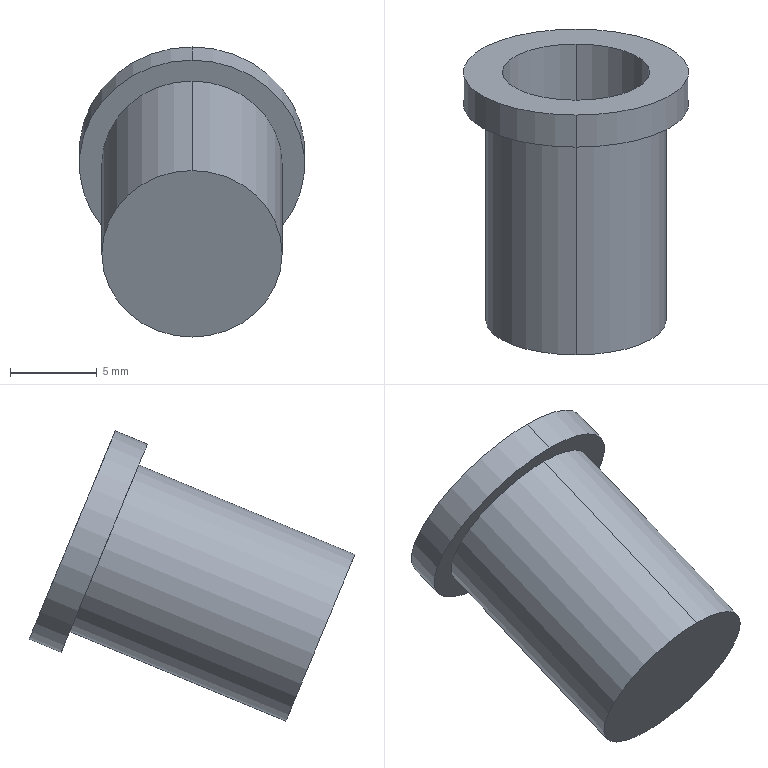Part | STEP file | ADMI9201SOYF_11_1 | 1 solid | 10 faces | box 13 x 18.798 x 16.741 mm | volume 788.076 mm3 | cylinder 6 | plane 4 | commonest cylinder face diameters 8.5 x2 10.4 x2 13 x2
STEP:
#1=CARTESIAN_POINT('',(2623.992,-732.037,12.183));
#2=VERTEX_POINT('',#1);
#3=CARTESIAN_POINT('',(2623.992,-736.017,21.791));
#4=VERTEX_POINT('',#3);
#5=CARTESIAN_POINT('',(2623.992,-734.027,16.987));
#6=DIRECTION('',(0.,-0.9239,-0.3827));
#7=DIRECTION('',(0.,0.3827,-0.9239));
#8=AXIS2_PLACEMENT_3D('',#5,#6,#7);
#9=CIRCLE('',#8,5.2);
#10=EDGE_CURVE('',#2,#4,#9,.T.);
#11=ORIENTED_EDGE('',*,*,#10,.T.);
#12=CARTESIAN_POINT('',(2623.992,-748.489,16.625));
#13=VERTEX_POINT('',#12);
#14=CARTESIAN_POINT('',(2623.992,-736.017,21.791));
#15=DIRECTION('',(0.,-0.9239,-0.3827));
#16=VECTOR('',#15,1000.);
#17=LINE('',#14,#16);
#18=EDGE_CURVE('',#4,#13,#17,.T.);
#19=ORIENTED_EDGE('',*,*,#18,.T.);
#20=CARTESIAN_POINT('',(2623.992,-744.51,7.016));
#21=VERTEX_POINT('',#20);
#22=CARTESIAN_POINT('',(2623.992,-746.499,11.821));
#23=DIRECTION('',(0.,0.9239,0.3827));
#24=DIRECTION('',(0.,0.3827,-0.9239));
#25=AXIS2_PLACEMENT_3D('',#22,#23,#24);
#26=CIRCLE('',#25,5.2);
#27=EDGE_CURVE('',#13,#21,#26,.T.);
#28=ORIENTED_EDGE('',*,*,#27,.T.);
#29=CARTESIAN_POINT('',(2623.992,-732.037,12.183));
#30=DIRECTION('',(0.,-0.9239,-0.3827));
#31=VECTOR('',#30,1000.);
#32=LINE('',#29,#31);
#33=EDGE_CURVE('',#2,#21,#32,.T.);
#34=ORIENTED_EDGE('',*,*,#33,.F.);
#35=EDGE_LOOP('',(#11,#19,#28,#34));
#36=FACE_OUTER_BOUND('',#35,.T.);
#37=CARTESIAN_POINT('',(2623.992,-734.027,16.987));
#38=DIRECTION('',(0.,-0.9239,-0.3827));
#39=DIRECTION('',(0.,0.3827,-0.9239));
#40=AXIS2_PLACEMENT_3D('',#37,#38,#39);
#41=CYLINDRICAL_SURFACE('',#40,5.2);
#42=ADVANCED_FACE('',(#36),#41,.T.);
#43=CARTESIAN_POINT('',(2623.992,-729.692,11.747));
#44=VERTEX_POINT('',#43);
#45=CARTESIAN_POINT('',(2623.992,-734.667,23.757));
#46=VERTEX_POINT('',#45);
#47=CARTESIAN_POINT('',(2623.992,-732.179,17.752));
#48=DIRECTION('',(0.,-0.9239,-0.3827));
#49=DIRECTION('',(0.,0.3827,-0.9239));
#50=AXIS2_PLACEMENT_3D('',#47,#48,#49);
#51=CIRCLE('',#50,6.5);
#52=EDGE_CURVE('',#44,#46,#51,.T.);
#53=ORIENTED_EDGE('',*,*,#52,.T.);
#54=CARTESIAN_POINT('',(2623.992,-736.515,22.992));
#55=VERTEX_POINT('',#54);
#56=CARTESIAN_POINT('',(2623.992,-734.667,23.757));
#57=DIRECTION('',(0.,-0.9239,-0.3827));
#58=VECTOR('',#57,1000.);
#59=LINE('',#56,#58);
#60=EDGE_CURVE('',#46,#55,#59,.T.);
#61=ORIENTED_EDGE('',*,*,#60,.T.);
#62=CARTESIAN_POINT('',(2623.992,-731.54,10.982));
#63=VERTEX_POINT('',#62);
#64=CARTESIAN_POINT('',(2623.992,-734.027,16.987));
#65=DIRECTION('',(0.,0.9239,0.3827));
#66=DIRECTION('',(0.,0.3827,-0.9239));
#67=AXIS2_PLACEMENT_3D('',#64,#65,#66);
#68=CIRCLE('',#67,6.5);
#69=EDGE_CURVE('',#55,#63,#68,.T.);
#70=ORIENTED_EDGE('',*,*,#69,.T.);
#71=CARTESIAN_POINT('',(2623.992,-729.692,11.747));
#72=DIRECTION('',(0.,-0.9239,-0.3827));
#73=VECTOR('',#72,1000.);
#74=LINE('',#71,#73);
#75=EDGE_CURVE('',#44,#63,#74,.T.);
#76=ORIENTED_EDGE('',*,*,#75,.F.);
#77=EDGE_LOOP('',(#53,#61,#70,#76));
#78=FACE_OUTER_BOUND('',#77,.T.);
#79=CARTESIAN_POINT('',(2623.992,-732.179,17.752));
#80=DIRECTION('',(0.,-0.9239,-0.3827));
#81=DIRECTION('',(0.,0.3827,-0.9239));
#82=AXIS2_PLACEMENT_3D('',#79,#80,#81);
#83=CYLINDRICAL_SURFACE('',#82,6.5);
#84=ADVANCED_FACE('',(#78),#83,.T.);
#85=CARTESIAN_POINT('',(2623.992,-740.716,9.616));
#86=VERTEX_POINT('',#85);
#87=CARTESIAN_POINT('',(2623.992,-743.968,17.469));
#88=VERTEX_POINT('',#87);
#89=CARTESIAN_POINT('',(2623.992,-742.342,13.543));
#90=DIRECTION('',(0.,0.9239,0.3827));
#91=DIRECTION('',(0.,-0.3827,0.9239));
#92=AXIS2_PLACEMENT_3D('',#89,#90,#91);
#93=CIRCLE('',#92,4.25);
#94=EDGE_CURVE('',#86,#88,#93,.T.);
#95=ORIENTED_EDGE('',*,*,#94,.F.);
#96=CARTESIAN_POINT('',(2623.992,-730.553,13.826));
#97=VERTEX_POINT('',#96);
#98=CARTESIAN_POINT('',(2623.992,-740.716,9.616));
#99=DIRECTION('',(0.,0.9239,0.3827));
#100=VECTOR('',#99,1000.);
#101=LINE('',#98,#100);
#102=EDGE_CURVE('',#86,#97,#101,.T.);
#103=ORIENTED_EDGE('',*,*,#102,.T.);
#104=CARTESIAN_POINT('',(2623.992,-733.806,21.679));
#105=VERTEX_POINT('',#104);
#106=CARTESIAN_POINT('',(2623.992,-732.179,17.752));
#107=DIRECTION('',(0.,-0.9239,-0.3827));
#108=DIRECTION('',(0.,-0.3827,0.9239));
#109=AXIS2_PLACEMENT_3D('',#106,#107,#108);
#110=CIRCLE('',#109,4.25);
#111=EDGE_CURVE('',#105,#97,#110,.T.);
#112=ORIENTED_EDGE('',*,*,#111,.F.);
#113=CARTESIAN_POINT('',(2623.992,-743.968,17.469));
#114=DIRECTION('',(0.,0.9239,0.3827));
#115=VECTOR('',#114,1000.);
#116=LINE('',#113,#115);
#117=EDGE_CURVE('',#88,#105,#116,.T.);
#118=ORIENTED_EDGE('',*,*,#117,.F.);
#119=EDGE_LOOP('',(#95,#103,#112,#118));
#120=FACE_OUTER_BOUND('',#119,.T.);
#121=CARTESIAN_POINT('',(2623.992,-742.342,13.543));
#122=DIRECTION('',(0.,0.9239,0.3827));
#123=DIRECTION('',(0.,-0.3827,0.9239));
#124=AXIS2_PLACEMENT_3D('',#121,#122,#123);
#125=CYLINDRICAL_SURFACE('',#124,4.25);
#126=ADVANCED_FACE('',(#120),#125,.F.);
#127=ORIENTED_EDGE('',*,*,#18,.F.);
#128=CARTESIAN_POINT('',(2623.992,-734.027,16.987));
#129=DIRECTION('',(0.,-0.9239,-0.3827));
#130=DIRECTION('',(0.,0.3827,-0.9239));
#131=AXIS2_PLACEMENT_3D('',#128,#129,#130);
#132=CIRCLE('',#131,5.2);
#133=EDGE_CURVE('',#4,#2,#132,.T.);
#134=ORIENTED_EDGE('',*,*,#133,.T.);
#135=ORIENTED_EDGE('',*,*,#33,.T.);
#136=CARTESIAN_POINT('',(2623.992,-746.499,11.821));
#137=DIRECTION('',(0.,0.9239,0.3827));
#138=DIRECTION('',(0.,0.3827,-0.9239));
#139=AXIS2_PLACEMENT_3D('',#136,#137,#138);
#140=CIRCLE('',#139,5.2);
#141=EDGE_CURVE('',#21,#13,#140,.T.);
#142=ORIENTED_EDGE('',*,*,#141,.T.);
#143=EDGE_LOOP('',(#127,#134,#135,#142));
#144=FACE_OUTER_BOUND('',#143,.T.);
#145=CARTESIAN_POINT('',(2623.992,-734.027,16.987));
#146=DIRECTION('',(0.,-0.9239,-0.3827));
#147=DIRECTION('',(0.,0.3827,-0.9239));
#148=AXIS2_PLACEMENT_3D('',#145,#146,#147);
#149=CYLINDRICAL_SURFACE('',#148,5.2);
#150=ADVANCED_FACE('',(#144),#149,.T.);
#151=ORIENTED_EDGE('',*,*,#10,.F.);
#152=ORIENTED_EDGE('',*,*,#133,.F.);
#153=EDGE_LOOP('',(#151,#152));
#154=FACE_BOUND('',#153,.T.);
#155=CARTESIAN_POINT('',(2623.992,-734.027,16.987));
#156=DIRECTION('',(0.,0.9239,0.3827));
#157=DIRECTION('',(0.,0.3827,-0.9239));
#158=AXIS2_PLACEMENT_3D('',#155,#156,#157);
#159=CIRCLE('',#158,6.5);
#160=EDGE_CURVE('',#63,#55,#159,.T.);
#161=ORIENTED_EDGE('',*,*,#160,.F.);
#162=ORIENTED_EDGE('',*,*,#69,.F.);
#163=EDGE_LOOP('',(#161,#162));
#164=FACE_OUTER_BOUND('',#163,.T.);
#165=CARTESIAN_POINT('',(2623.992,-734.027,16.987));
#166=DIRECTION('',(0.,0.9239,0.3827));
#167=DIRECTION('',(0.,-0.3827,0.9239));
#168=AXIS2_PLACEMENT_3D('',#165,#166,#167);
#169=PLANE('',#168);
#170=ADVANCED_FACE('',(#154,#164),#169,.F.);
#171=ORIENTED_EDGE('',*,*,#141,.F.);
#172=ORIENTED_EDGE('',*,*,#27,.F.);
#173=EDGE_LOOP('',(#171,#172));
#174=FACE_OUTER_BOUND('',#173,.T.);
#175=CARTESIAN_POINT('',(2623.992,-746.499,11.821));
#176=DIRECTION('',(0.,0.9239,0.3827));
#177=DIRECTION('',(0.,-0.3827,0.9239));
#178=AXIS2_PLACEMENT_3D('',#175,#176,#177);
#179=PLANE('',#178);
#180=ADVANCED_FACE('',(#174),#179,.F.);
#181=ORIENTED_EDGE('',*,*,#60,.F.);
#182=CARTESIAN_POINT('',(2623.992,-732.179,17.752));
#183=DIRECTION('',(0.,-0.9239,-0.3827));
#184=DIRECTION('',(0.,0.3827,-0.9239));
#185=AXIS2_PLACEMENT_3D('',#182,#183,#184);
#186=CIRCLE('',#185,6.5);
#187=EDGE_CURVE('',#46,#44,#186,.T.);
#188=ORIENTED_EDGE('',*,*,#187,.T.);
#189=ORIENTED_EDGE('',*,*,#75,.T.);
#190=ORIENTED_EDGE('',*,*,#160,.T.);
#191=EDGE_LOOP('',(#181,#188,#189,#190));
#192=FACE_OUTER_BOUND('',#191,.T.);
#193=CARTESIAN_POINT('',(2623.992,-732.179,17.752));
#194=DIRECTION('',(0.,-0.9239,-0.3827));
#195=DIRECTION('',(0.,0.3827,-0.9239));
#196=AXIS2_PLACEMENT_3D('',#193,#194,#195);
#197=CYLINDRICAL_SURFACE('',#196,6.5);
#198=ADVANCED_FACE('',(#192),#197,.T.);
#199=ORIENTED_EDGE('',*,*,#111,.T.);
#200=CARTESIAN_POINT('',(2623.992,-732.179,17.752));
#201=DIRECTION('',(0.,-0.9239,-0.3827));
#202=DIRECTION('',(0.,-0.3827,0.9239));
#203=AXIS2_PLACEMENT_3D('',#200,#201,#202);
#204=CIRCLE('',#203,4.25);
#205=EDGE_CURVE('',#97,#105,#204,.T.);
#206=ORIENTED_EDGE('',*,*,#205,.T.);
#207=EDGE_LOOP('',(#199,#206));
#208=FACE_BOUND('',#207,.T.);
#209=ORIENTED_EDGE('',*,*,#52,.F.);
#210=ORIENTED_EDGE('',*,*,#187,.F.);
#211=EDGE_LOOP('',(#209,#210));
#212=FACE_OUTER_BOUND('',#211,.T.);
#213=CARTESIAN_POINT('',(2623.992,-732.179,17.752));
#214=DIRECTION('',(0.,0.9239,0.3827));
#215=DIRECTION('',(0.,-0.3827,0.9239));
#216=AXIS2_PLACEMENT_3D('',#213,#214,#215);
#217=PLANE('',#216);
#218=ADVANCED_FACE('',(#208,#212),#217,.T.);
#219=ORIENTED_EDGE('',*,*,#102,.F.);
#220=CARTESIAN_POINT('',(2623.992,-742.342,13.543));
#221=DIRECTION('',(0.,0.9239,0.3827));
#222=DIRECTION('',(0.,-0.3827,0.9239));
#223=AXIS2_PLACEMENT_3D('',#220,#221,#222);
#224=CIRCLE('',#223,4.25);
#225=EDGE_CURVE('',#88,#86,#224,.T.);
#226=ORIENTED_EDGE('',*,*,#225,.F.);
#227=ORIENTED_EDGE('',*,*,#117,.T.);
#228=ORIENTED_EDGE('',*,*,#205,.F.);
#229=EDGE_LOOP('',(#219,#226,#227,#228));
#230=FACE_OUTER_BOUND('',#229,.T.);
#231=CARTESIAN_POINT('',(2623.992,-742.342,13.543));
#232=DIRECTION('',(0.,0.9239,0.3827));
#233=DIRECTION('',(0.,-0.3827,0.9239));
#234=AXIS2_PLACEMENT_3D('',#231,#232,#233);
#235=CYLINDRICAL_SURFACE('',#234,4.25);
#236=ADVANCED_FACE('',(#230),#235,.F.);
#237=ORIENTED_EDGE('',*,*,#225,.T.);
#238=ORIENTED_EDGE('',*,*,#94,.T.);
#239=EDGE_LOOP('',(#237,#238));
#240=FACE_OUTER_BOUND('',#239,.T.);
#241=CARTESIAN_POINT('',(2623.992,-742.342,13.543));
#242=DIRECTION('',(0.,0.9239,0.3827));
#243=DIRECTION('',(0.,-0.3827,0.9239));
#244=AXIS2_PLACEMENT_3D('',#241,#242,#243);
#245=PLANE('',#244);
#246=ADVANCED_FACE('',(#240),#245,.T.);
#247=CLOSED_SHELL('',(#42,#84,#126,#150,#170,#180,#198,#218,#236,#246));
#248=MANIFOLD_SOLID_BREP('',#247);
#249=CARTESIAN_POINT('',(0.,0.,0.));
#250=DIRECTION('',(0.,0.,1.));
#251=DIRECTION('',(1.,0.,0.));
#252=AXIS2_PLACEMENT_3D('',#249,#250,#251);
#253=(LENGTH_UNIT()NAMED_UNIT(*)SI_UNIT(.MILLI.,.METRE.));
#254=UNCERTAINTY_MEASURE_WITH_UNIT(LENGTH_MEASURE(0.00001),#253,'','');
#255=(NAMED_UNIT(*)PLANE_ANGLE_UNIT()SI_UNIT($,.RADIAN.));
#256=(NAMED_UNIT(*)SI_UNIT($,.STERADIAN.)SOLID_ANGLE_UNIT());
#257=(GEOMETRIC_REPRESENTATION_CONTEXT(3)GLOBAL_UNCERTAINTY_ASSIGNED_CONTEXT((#254))GLOBAL_UNIT_ASSIGNED_CONTEXT((#253,#255,#256))REPRESENTATION_CONTEXT('',''));
#258=ADVANCED_BREP_SHAPE_REPRESENTATION('',(#248,#252),#257);